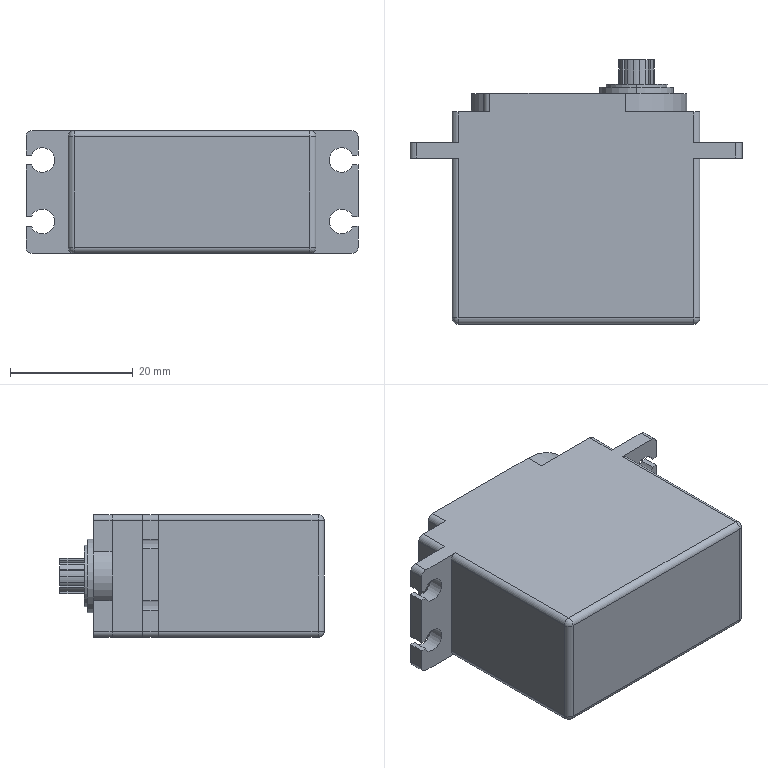Part | SolidWorks | features ICE 5, 3DProfileFeature 1, Extrusion 1, Fillet 1, HoleWzd 1 | 1 solid | 108 faces | box 54 x 43 x 20 mm | volume 30390 mm3 | cylinder 51 | plane 51 | sphere 4 | cone 2 | commonest cylinder face diameters 2 x18 5.8 x10 5 x9 4 x6 10 x3 2.5 x2